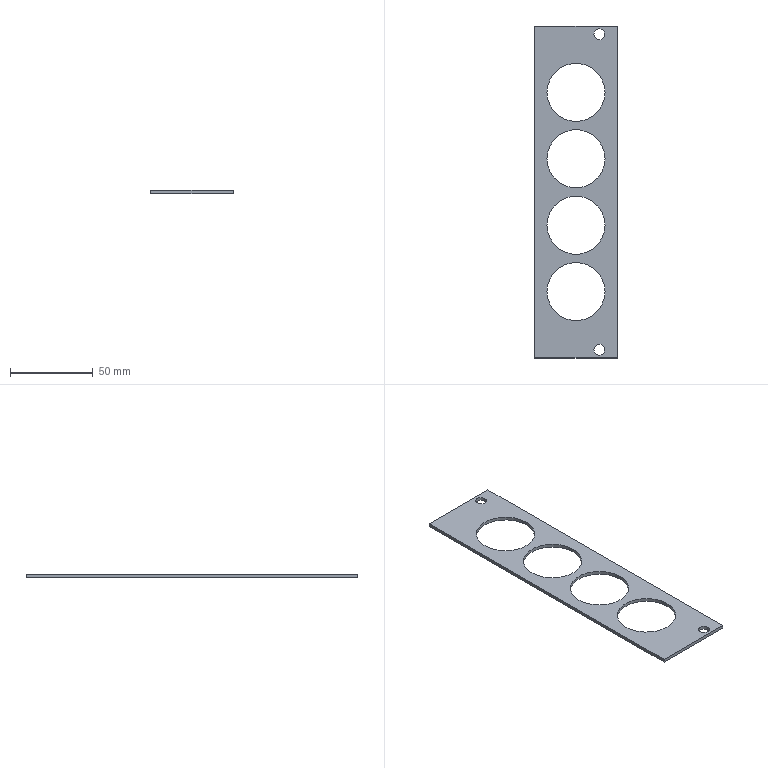Part | SolidWorks | features BaseBody 1 | 1 solid | 18 faces | box 50 x 200 x 2 mm | volume 12170 mm3 | cylinder 12 | plane 6 | commonest cylinder face diameters 35 x8 6.5 x4
STEP:
#1=CARTESIAN_POINT('',(175.446,-4210.973,117.471));
#2=VERTEX_POINT('',#1);
#3=CARTESIAN_POINT('',(210.446,-4210.973,117.471));
#4=VERTEX_POINT('',#3);
#5=CARTESIAN_POINT('',(192.946,-4210.973,117.471));
#6=DIRECTION('',(0.,0.,1.));
#7=DIRECTION('',(1.,0.,0.));
#8=AXIS2_PLACEMENT_3D('',#5,#6,#7);
#9=CIRCLE('',#8,17.5);
#10=EDGE_CURVE('',#2,#4,#9,.T.);
#11=ORIENTED_EDGE('',*,*,#10,.F.);
#12=CARTESIAN_POINT('',(175.446,-4210.973,119.471));
#13=VERTEX_POINT('',#12);
#14=CARTESIAN_POINT('',(175.446,-4210.973,120.383));
#15=DIRECTION('',(0.,0.,1.));
#16=VECTOR('',#15,1000.);
#17=LINE('',#14,#16);
#18=EDGE_CURVE('',#2,#13,#17,.T.);
#19=ORIENTED_EDGE('',*,*,#18,.T.);
#20=CARTESIAN_POINT('',(210.446,-4210.973,119.471));
#21=VERTEX_POINT('',#20);
#22=CARTESIAN_POINT('',(192.946,-4210.973,119.471));
#23=DIRECTION('',(0.,0.,-1.));
#24=DIRECTION('',(1.,0.,0.));
#25=AXIS2_PLACEMENT_3D('',#22,#23,#24);
#26=CIRCLE('',#25,17.5);
#27=EDGE_CURVE('',#21,#13,#26,.T.);
#28=ORIENTED_EDGE('',*,*,#27,.F.);
#29=CARTESIAN_POINT('',(210.446,-4210.973,120.383));
#30=DIRECTION('',(0.,0.,1.));
#31=VECTOR('',#30,1000.);
#32=LINE('',#29,#31);
#33=EDGE_CURVE('',#4,#21,#32,.T.);
#34=ORIENTED_EDGE('',*,*,#33,.F.);
#35=EDGE_LOOP('',(#11,#19,#28,#34));
#36=FACE_OUTER_BOUND('',#35,.T.);
#37=CARTESIAN_POINT('',(192.946,-4210.973,120.383));
#38=DIRECTION('',(0.,0.,1.));
#39=DIRECTION('',(1.,0.,0.));
#40=AXIS2_PLACEMENT_3D('',#37,#38,#39);
#41=CYLINDRICAL_SURFACE('',#40,17.5);
#42=ADVANCED_FACE('',(#36),#41,.F.);
#43=CARTESIAN_POINT('',(210.446,-4250.973,119.471));
#44=VERTEX_POINT('',#43);
#45=CARTESIAN_POINT('',(175.446,-4250.973,119.471));
#46=VERTEX_POINT('',#45);
#47=CARTESIAN_POINT('',(192.946,-4250.973,119.471));
#48=DIRECTION('',(0.,0.,-1.));
#49=DIRECTION('',(-1.,0.,0.));
#50=AXIS2_PLACEMENT_3D('',#47,#48,#49);
#51=CIRCLE('',#50,17.5);
#52=EDGE_CURVE('',#44,#46,#51,.T.);
#53=ORIENTED_EDGE('',*,*,#52,.F.);
#54=CARTESIAN_POINT('',(210.446,-4250.973,117.471));
#55=VERTEX_POINT('',#54);
#56=CARTESIAN_POINT('',(210.446,-4250.973,120.383));
#57=DIRECTION('',(0.,0.,-1.));
#58=VECTOR('',#57,1000.);
#59=LINE('',#56,#58);
#60=EDGE_CURVE('',#44,#55,#59,.T.);
#61=ORIENTED_EDGE('',*,*,#60,.T.);
#62=CARTESIAN_POINT('',(175.446,-4250.973,117.471));
#63=VERTEX_POINT('',#62);
#64=CARTESIAN_POINT('',(192.946,-4250.973,117.471));
#65=DIRECTION('',(0.,0.,1.));
#66=DIRECTION('',(-1.,0.,0.));
#67=AXIS2_PLACEMENT_3D('',#64,#65,#66);
#68=CIRCLE('',#67,17.5);
#69=EDGE_CURVE('',#63,#55,#68,.T.);
#70=ORIENTED_EDGE('',*,*,#69,.F.);
#71=CARTESIAN_POINT('',(175.446,-4250.973,120.383));
#72=DIRECTION('',(0.,0.,-1.));
#73=VECTOR('',#72,1000.);
#74=LINE('',#71,#73);
#75=EDGE_CURVE('',#46,#63,#74,.T.);
#76=ORIENTED_EDGE('',*,*,#75,.F.);
#77=EDGE_LOOP('',(#53,#61,#70,#76));
#78=FACE_OUTER_BOUND('',#77,.T.);
#79=CARTESIAN_POINT('',(192.946,-4250.973,120.383));
#80=DIRECTION('',(0.,0.,-1.));
#81=DIRECTION('',(-1.,0.,0.));
#82=AXIS2_PLACEMENT_3D('',#79,#80,#81);
#83=CYLINDRICAL_SURFACE('',#82,17.5);
#84=ADVANCED_FACE('',(#78),#83,.F.);
#85=CARTESIAN_POINT('',(203.696,-4135.973,117.471));
#86=VERTEX_POINT('',#85);
#87=CARTESIAN_POINT('',(210.196,-4135.973,117.471));
#88=VERTEX_POINT('',#87);
#89=CARTESIAN_POINT('',(206.946,-4135.973,117.471));
#90=DIRECTION('',(0.,0.,1.));
#91=DIRECTION('',(1.,0.,0.));
#92=AXIS2_PLACEMENT_3D('',#89,#90,#91);
#93=CIRCLE('',#92,3.25);
#94=EDGE_CURVE('',#86,#88,#93,.T.);
#95=ORIENTED_EDGE('',*,*,#94,.F.);
#96=CARTESIAN_POINT('',(203.696,-4135.973,119.471));
#97=VERTEX_POINT('',#96);
#98=CARTESIAN_POINT('',(203.696,-4135.973,120.383));
#99=DIRECTION('',(0.,0.,1.));
#100=VECTOR('',#99,1000.);
#101=LINE('',#98,#100);
#102=EDGE_CURVE('',#86,#97,#101,.T.);
#103=ORIENTED_EDGE('',*,*,#102,.T.);
#104=CARTESIAN_POINT('',(210.196,-4135.973,119.471));
#105=VERTEX_POINT('',#104);
#106=CARTESIAN_POINT('',(206.946,-4135.973,119.471));
#107=DIRECTION('',(0.,0.,-1.));
#108=DIRECTION('',(1.,0.,0.));
#109=AXIS2_PLACEMENT_3D('',#106,#107,#108);
#110=CIRCLE('',#109,3.25);
#111=EDGE_CURVE('',#105,#97,#110,.T.);
#112=ORIENTED_EDGE('',*,*,#111,.F.);
#113=CARTESIAN_POINT('',(210.196,-4135.973,120.383));
#114=DIRECTION('',(0.,0.,1.));
#115=VECTOR('',#114,1000.);
#116=LINE('',#113,#115);
#117=EDGE_CURVE('',#88,#105,#116,.T.);
#118=ORIENTED_EDGE('',*,*,#117,.F.);
#119=EDGE_LOOP('',(#95,#103,#112,#118));
#120=FACE_OUTER_BOUND('',#119,.T.);
#121=CARTESIAN_POINT('',(206.946,-4135.973,120.383));
#122=DIRECTION('',(0.,0.,1.));
#123=DIRECTION('',(1.,0.,0.));
#124=AXIS2_PLACEMENT_3D('',#121,#122,#123);
#125=CYLINDRICAL_SURFACE('',#124,3.25);
#126=ADVANCED_FACE('',(#120),#125,.F.);
#127=CARTESIAN_POINT('',(210.196,-4325.973,119.471));
#128=VERTEX_POINT('',#127);
#129=CARTESIAN_POINT('',(203.696,-4325.973,119.471));
#130=VERTEX_POINT('',#129);
#131=CARTESIAN_POINT('',(206.946,-4325.973,119.471));
#132=DIRECTION('',(0.,0.,-1.));
#133=DIRECTION('',(-1.,0.,0.));
#134=AXIS2_PLACEMENT_3D('',#131,#132,#133);
#135=CIRCLE('',#134,3.25);
#136=EDGE_CURVE('',#128,#130,#135,.T.);
#137=ORIENTED_EDGE('',*,*,#136,.F.);
#138=CARTESIAN_POINT('',(210.196,-4325.973,117.471));
#139=VERTEX_POINT('',#138);
#140=CARTESIAN_POINT('',(210.196,-4325.973,120.383));
#141=DIRECTION('',(0.,0.,-1.));
#142=VECTOR('',#141,1000.);
#143=LINE('',#140,#142);
#144=EDGE_CURVE('',#128,#139,#143,.T.);
#145=ORIENTED_EDGE('',*,*,#144,.T.);
#146=CARTESIAN_POINT('',(203.696,-4325.973,117.471));
#147=VERTEX_POINT('',#146);
#148=CARTESIAN_POINT('',(206.946,-4325.973,117.471));
#149=DIRECTION('',(0.,0.,1.));
#150=DIRECTION('',(-1.,0.,0.));
#151=AXIS2_PLACEMENT_3D('',#148,#149,#150);
#152=CIRCLE('',#151,3.25);
#153=EDGE_CURVE('',#147,#139,#152,.T.);
#154=ORIENTED_EDGE('',*,*,#153,.F.);
#155=CARTESIAN_POINT('',(203.696,-4325.973,120.383));
#156=DIRECTION('',(0.,0.,-1.));
#157=VECTOR('',#156,1000.);
#158=LINE('',#155,#157);
#159=EDGE_CURVE('',#130,#147,#158,.T.);
#160=ORIENTED_EDGE('',*,*,#159,.F.);
#161=EDGE_LOOP('',(#137,#145,#154,#160));
#162=FACE_OUTER_BOUND('',#161,.T.);
#163=CARTESIAN_POINT('',(206.946,-4325.973,120.383));
#164=DIRECTION('',(0.,0.,-1.));
#165=DIRECTION('',(-1.,0.,0.));
#166=AXIS2_PLACEMENT_3D('',#163,#164,#165);
#167=CYLINDRICAL_SURFACE('',#166,3.25);
#168=ADVANCED_FACE('',(#162),#167,.F.);
#169=CARTESIAN_POINT('',(210.446,-4290.973,119.471));
#170=VERTEX_POINT('',#169);
#171=CARTESIAN_POINT('',(175.446,-4290.973,119.471));
#172=VERTEX_POINT('',#171);
#173=CARTESIAN_POINT('',(192.946,-4290.973,119.471));
#174=DIRECTION('',(0.,0.,-1.));
#175=DIRECTION('',(-1.,0.,0.));
#176=AXIS2_PLACEMENT_3D('',#173,#174,#175);
#177=CIRCLE('',#176,17.5);
#178=EDGE_CURVE('',#170,#172,#177,.T.);
#179=ORIENTED_EDGE('',*,*,#178,.F.);
#180=CARTESIAN_POINT('',(210.446,-4290.973,117.471));
#181=VERTEX_POINT('',#180);
#182=CARTESIAN_POINT('',(210.446,-4290.973,120.383));
#183=DIRECTION('',(0.,0.,-1.));
#184=VECTOR('',#183,1000.);
#185=LINE('',#182,#184);
#186=EDGE_CURVE('',#170,#181,#185,.T.);
#187=ORIENTED_EDGE('',*,*,#186,.T.);
#188=CARTESIAN_POINT('',(175.446,-4290.973,117.471));
#189=VERTEX_POINT('',#188);
#190=CARTESIAN_POINT('',(192.946,-4290.973,117.471));
#191=DIRECTION('',(0.,0.,1.));
#192=DIRECTION('',(-1.,0.,0.));
#193=AXIS2_PLACEMENT_3D('',#190,#191,#192);
#194=CIRCLE('',#193,17.5);
#195=EDGE_CURVE('',#189,#181,#194,.T.);
#196=ORIENTED_EDGE('',*,*,#195,.F.);
#197=CARTESIAN_POINT('',(175.446,-4290.973,120.383));
#198=DIRECTION('',(0.,0.,-1.));
#199=VECTOR('',#198,1000.);
#200=LINE('',#197,#199);
#201=EDGE_CURVE('',#172,#189,#200,.T.);
#202=ORIENTED_EDGE('',*,*,#201,.F.);
#203=EDGE_LOOP('',(#179,#187,#196,#202));
#204=FACE_OUTER_BOUND('',#203,.T.);
#205=CARTESIAN_POINT('',(192.946,-4290.973,120.383));
#206=DIRECTION('',(0.,0.,-1.));
#207=DIRECTION('',(-1.,0.,0.));
#208=AXIS2_PLACEMENT_3D('',#205,#206,#207);
#209=CYLINDRICAL_SURFACE('',#208,17.5);
#210=ADVANCED_FACE('',(#204),#209,.F.);
#211=CARTESIAN_POINT('',(175.446,-4170.973,117.471));
#212=VERTEX_POINT('',#211);
#213=CARTESIAN_POINT('',(210.446,-4170.973,117.471));
#214=VERTEX_POINT('',#213);
#215=CARTESIAN_POINT('',(192.946,-4170.973,117.471));
#216=DIRECTION('',(0.,0.,1.));
#217=DIRECTION('',(1.,0.,0.));
#218=AXIS2_PLACEMENT_3D('',#215,#216,#217);
#219=CIRCLE('',#218,17.5);
#220=EDGE_CURVE('',#212,#214,#219,.T.);
#221=ORIENTED_EDGE('',*,*,#220,.F.);
#222=CARTESIAN_POINT('',(175.446,-4170.973,119.471));
#223=VERTEX_POINT('',#222);
#224=CARTESIAN_POINT('',(175.446,-4170.973,120.383));
#225=DIRECTION('',(0.,0.,1.));
#226=VECTOR('',#225,1000.);
#227=LINE('',#224,#226);
#228=EDGE_CURVE('',#212,#223,#227,.T.);
#229=ORIENTED_EDGE('',*,*,#228,.T.);
#230=CARTESIAN_POINT('',(210.446,-4170.973,119.471));
#231=VERTEX_POINT('',#230);
#232=CARTESIAN_POINT('',(192.946,-4170.973,119.471));
#233=DIRECTION('',(0.,0.,-1.));
#234=DIRECTION('',(1.,0.,0.));
#235=AXIS2_PLACEMENT_3D('',#232,#233,#234);
#236=CIRCLE('',#235,17.5);
#237=EDGE_CURVE('',#231,#223,#236,.T.);
#238=ORIENTED_EDGE('',*,*,#237,.F.);
#239=CARTESIAN_POINT('',(210.446,-4170.973,120.383));
#240=DIRECTION('',(0.,0.,1.));
#241=VECTOR('',#240,1000.);
#242=LINE('',#239,#241);
#243=EDGE_CURVE('',#214,#231,#242,.T.);
#244=ORIENTED_EDGE('',*,*,#243,.F.);
#245=EDGE_LOOP('',(#221,#229,#238,#244));
#246=FACE_OUTER_BOUND('',#245,.T.);
#247=CARTESIAN_POINT('',(192.946,-4170.973,120.383));
#248=DIRECTION('',(0.,0.,1.));
#249=DIRECTION('',(1.,0.,0.));
#250=AXIS2_PLACEMENT_3D('',#247,#248,#249);
#251=CYLINDRICAL_SURFACE('',#250,17.5);
#252=ADVANCED_FACE('',(#246),#251,.F.);
#253=CARTESIAN_POINT('',(167.946,-4330.973,119.471));
#254=VERTEX_POINT('',#253);
#255=CARTESIAN_POINT('',(217.946,-4330.973,119.471));
#256=VERTEX_POINT('',#255);
#257=CARTESIAN_POINT('',(192.946,-4330.973,119.471));
#258=DIRECTION('',(1.,0.,0.));
#259=VECTOR('',#258,1000.);
#260=LINE('',#257,#259);
#261=EDGE_CURVE('',#254,#256,#260,.T.);
#262=ORIENTED_EDGE('',*,*,#261,.T.);
#263=CARTESIAN_POINT('',(217.946,-4130.973,119.471));
#264=VERTEX_POINT('',#263);
#265=CARTESIAN_POINT('',(217.946,-4230.973,119.471));
#266=DIRECTION('',(0.,1.,0.));
#267=VECTOR('',#266,1000.);
#268=LINE('',#265,#267);
#269=EDGE_CURVE('',#256,#264,#268,.T.);
#270=ORIENTED_EDGE('',*,*,#269,.T.);
#271=CARTESIAN_POINT('',(167.946,-4130.973,119.471));
#272=VERTEX_POINT('',#271);
#273=CARTESIAN_POINT('',(192.946,-4130.973,119.471));
#274=DIRECTION('',(-1.,0.,0.));
#275=VECTOR('',#274,1000.);
#276=LINE('',#273,#275);
#277=EDGE_CURVE('',#264,#272,#276,.T.);
#278=ORIENTED_EDGE('',*,*,#277,.T.);
#279=CARTESIAN_POINT('',(167.946,-4230.973,119.471));
#280=DIRECTION('',(0.,-1.,0.));
#281=VECTOR('',#280,1000.);
#282=LINE('',#279,#281);
#283=EDGE_CURVE('',#272,#254,#282,.T.);
#284=ORIENTED_EDGE('',*,*,#283,.T.);
#285=EDGE_LOOP('',(#262,#270,#278,#284));
#286=FACE_OUTER_BOUND('',#285,.T.);
#287=ORIENTED_EDGE('',*,*,#27,.T.);
#288=CARTESIAN_POINT('',(192.946,-4210.973,119.471));
#289=DIRECTION('',(0.,0.,-1.));
#290=DIRECTION('',(1.,0.,0.));
#291=AXIS2_PLACEMENT_3D('',#288,#289,#290);
#292=CIRCLE('',#291,17.5);
#293=EDGE_CURVE('',#13,#21,#292,.T.);
#294=ORIENTED_EDGE('',*,*,#293,.T.);
#295=EDGE_LOOP('',(#287,#294));
#296=FACE_BOUND('',#295,.T.);
#297=CARTESIAN_POINT('',(192.946,-4250.973,119.471));
#298=DIRECTION('',(0.,0.,-1.));
#299=DIRECTION('',(-1.,0.,0.));
#300=AXIS2_PLACEMENT_3D('',#297,#298,#299);
#301=CIRCLE('',#300,17.5);
#302=EDGE_CURVE('',#46,#44,#301,.T.);
#303=ORIENTED_EDGE('',*,*,#302,.T.);
#304=ORIENTED_EDGE('',*,*,#52,.T.);
#305=EDGE_LOOP('',(#303,#304));
#306=FACE_BOUND('',#305,.T.);
#307=ORIENTED_EDGE('',*,*,#111,.T.);
#308=CARTESIAN_POINT('',(206.946,-4135.973,119.471));
#309=DIRECTION('',(0.,0.,-1.));
#310=DIRECTION('',(1.,0.,0.));
#311=AXIS2_PLACEMENT_3D('',#308,#309,#310);
#312=CIRCLE('',#311,3.25);
#313=EDGE_CURVE('',#97,#105,#312,.T.);
#314=ORIENTED_EDGE('',*,*,#313,.T.);
#315=EDGE_LOOP('',(#307,#314));
#316=FACE_BOUND('',#315,.T.);
#317=CARTESIAN_POINT('',(206.946,-4325.973,119.471));
#318=DIRECTION('',(0.,0.,-1.));
#319=DIRECTION('',(-1.,0.,0.));
#320=AXIS2_PLACEMENT_3D('',#317,#318,#319);
#321=CIRCLE('',#320,3.25);
#322=EDGE_CURVE('',#130,#128,#321,.T.);
#323=ORIENTED_EDGE('',*,*,#322,.T.);
#324=ORIENTED_EDGE('',*,*,#136,.T.);
#325=EDGE_LOOP('',(#323,#324));
#326=FACE_BOUND('',#325,.T.);
#327=CARTESIAN_POINT('',(192.946,-4290.973,119.471));
#328=DIRECTION('',(0.,0.,-1.));
#329=DIRECTION('',(-1.,0.,0.));
#330=AXIS2_PLACEMENT_3D('',#327,#328,#329);
#331=CIRCLE('',#330,17.5);
#332=EDGE_CURVE('',#172,#170,#331,.T.);
#333=ORIENTED_EDGE('',*,*,#332,.T.);
#334=ORIENTED_EDGE('',*,*,#178,.T.);
#335=EDGE_LOOP('',(#333,#334));
#336=FACE_BOUND('',#335,.T.);
#337=ORIENTED_EDGE('',*,*,#237,.T.);
#338=CARTESIAN_POINT('',(192.946,-4170.973,119.471));
#339=DIRECTION('',(0.,0.,-1.));
#340=DIRECTION('',(1.,0.,0.));
#341=AXIS2_PLACEMENT_3D('',#338,#339,#340);
#342=CIRCLE('',#341,17.5);
#343=EDGE_CURVE('',#223,#231,#342,.T.);
#344=ORIENTED_EDGE('',*,*,#343,.T.);
#345=EDGE_LOOP('',(#337,#344));
#346=FACE_BOUND('',#345,.T.);
#347=CARTESIAN_POINT('',(192.946,-4230.973,119.471));
#348=DIRECTION('',(0.,0.,1.));
#349=DIRECTION('',(1.,0.,0.));
#350=AXIS2_PLACEMENT_3D('',#347,#348,#349);
#351=PLANE('',#350);
#352=ADVANCED_FACE('',(#286,#296,#306,#316,#326,#336,#346),#351,.T.);
#353=CARTESIAN_POINT('',(217.946,-4330.973,117.471));
#354=VERTEX_POINT('',#353);
#355=CARTESIAN_POINT('',(217.946,-4130.973,117.471));
#356=VERTEX_POINT('',#355);
#357=CARTESIAN_POINT('',(217.946,-4130.973,117.471));
#358=DIRECTION('',(0.,1.,0.));
#359=VECTOR('',#358,1000.);
#360=LINE('',#357,#359);
#361=EDGE_CURVE('',#354,#356,#360,.T.);
#362=ORIENTED_EDGE('',*,*,#361,.T.);
#363=CARTESIAN_POINT('',(217.946,-4130.973,117.471));
#364=DIRECTION('',(0.,0.,1.));
#365=VECTOR('',#364,1000.);
#366=LINE('',#363,#365);
#367=EDGE_CURVE('',#356,#264,#366,.T.);
#368=ORIENTED_EDGE('',*,*,#367,.T.);
#369=ORIENTED_EDGE('',*,*,#269,.F.);
#370=CARTESIAN_POINT('',(217.946,-4330.973,117.471));
#371=DIRECTION('',(0.,0.,-1.));
#372=VECTOR('',#371,1000.);
#373=LINE('',#370,#372);
#374=EDGE_CURVE('',#256,#354,#373,.T.);
#375=ORIENTED_EDGE('',*,*,#374,.T.);
#376=EDGE_LOOP('',(#362,#368,#369,#375));
#377=FACE_OUTER_BOUND('',#376,.T.);
#378=CARTESIAN_POINT('',(217.946,-4130.973,117.471));
#379=DIRECTION('',(1.,0.,0.));
#380=DIRECTION('',(0.,0.,-1.));
#381=AXIS2_PLACEMENT_3D('',#378,#379,#380);
#382=PLANE('',#381);
#383=ADVANCED_FACE('',(#377),#382,.T.);
#384=CARTESIAN_POINT('',(167.946,-4330.973,117.471));
#385=VERTEX_POINT('',#384);
#386=CARTESIAN_POINT('',(217.946,-4330.973,117.471));
#387=DIRECTION('',(1.,0.,0.));
#388=VECTOR('',#387,1000.);
#389=LINE('',#386,#388);
#390=EDGE_CURVE('',#385,#354,#389,.T.);
#391=ORIENTED_EDGE('',*,*,#390,.T.);
#392=ORIENTED_EDGE('',*,*,#374,.F.);
#393=ORIENTED_EDGE('',*,*,#261,.F.);
#394=CARTESIAN_POINT('',(167.946,-4330.973,117.471));
#395=DIRECTION('',(0.,0.,-1.));
#396=VECTOR('',#395,1000.);
#397=LINE('',#394,#396);
#398=EDGE_CURVE('',#254,#385,#397,.T.);
#399=ORIENTED_EDGE('',*,*,#398,.T.);
#400=EDGE_LOOP('',(#391,#392,#393,#399));
#401=FACE_OUTER_BOUND('',#400,.T.);
#402=CARTESIAN_POINT('',(217.946,-4330.973,117.471));
#403=DIRECTION('',(0.,-1.,0.));
#404=DIRECTION('',(0.,0.,-1.));
#405=AXIS2_PLACEMENT_3D('',#402,#403,#404);
#406=PLANE('',#405);
#407=ADVANCED_FACE('',(#401),#406,.T.);
#408=CARTESIAN_POINT('',(167.946,-4130.973,117.471));
#409=VERTEX_POINT('',#408);
#410=CARTESIAN_POINT('',(167.946,-4330.973,117.471));
#411=DIRECTION('',(0.,-1.,0.));
#412=VECTOR('',#411,1000.);
#413=LINE('',#410,#412);
#414=EDGE_CURVE('',#409,#385,#413,.T.);
#415=ORIENTED_EDGE('',*,*,#414,.T.);
#416=ORIENTED_EDGE('',*,*,#398,.F.);
#417=ORIENTED_EDGE('',*,*,#283,.F.);
#418=CARTESIAN_POINT('',(167.946,-4130.973,117.471));
#419=DIRECTION('',(0.,0.,-1.));
#420=VECTOR('',#419,1000.);
#421=LINE('',#418,#420);
#422=EDGE_CURVE('',#272,#409,#421,.T.);
#423=ORIENTED_EDGE('',*,*,#422,.T.);
#424=EDGE_LOOP('',(#415,#416,#417,#423));
#425=FACE_OUTER_BOUND('',#424,.T.);
#426=CARTESIAN_POINT('',(167.946,-4330.973,117.471));
#427=DIRECTION('',(-1.,0.,0.));
#428=DIRECTION('',(0.,0.,1.));
#429=AXIS2_PLACEMENT_3D('',#426,#427,#428);
#430=PLANE('',#429);
#431=ADVANCED_FACE('',(#425),#430,.T.);
#432=CARTESIAN_POINT('',(167.946,-4130.973,117.471));
#433=DIRECTION('',(-1.,0.,0.));
#434=VECTOR('',#433,1000.);
#435=LINE('',#432,#434);
#436=EDGE_CURVE('',#356,#409,#435,.T.);
#437=ORIENTED_EDGE('',*,*,#436,.T.);
#438=ORIENTED_EDGE('',*,*,#422,.F.);
#439=ORIENTED_EDGE('',*,*,#277,.F.);
#440=ORIENTED_EDGE('',*,*,#367,.F.);
#441=EDGE_LOOP('',(#437,#438,#439,#440));
#442=FACE_OUTER_BOUND('',#441,.T.);
#443=CARTESIAN_POINT('',(167.946,-4130.973,117.471));
#444=DIRECTION('',(0.,1.,0.));
#445=DIRECTION('',(0.,0.,1.));
#446=AXIS2_PLACEMENT_3D('',#443,#444,#445);
#447=PLANE('',#446);
#448=ADVANCED_FACE('',(#442),#447,.T.);
#449=ORIENTED_EDGE('',*,*,#18,.F.);
#450=CARTESIAN_POINT('',(192.946,-4210.973,117.471));
#451=DIRECTION('',(0.,0.,1.));
#452=DIRECTION('',(1.,0.,0.));
#453=AXIS2_PLACEMENT_3D('',#450,#451,#452);
#454=CIRCLE('',#453,17.5);
#455=EDGE_CURVE('',#4,#2,#454,.T.);
#456=ORIENTED_EDGE('',*,*,#455,.F.);
#457=ORIENTED_EDGE('',*,*,#33,.T.);
#458=ORIENTED_EDGE('',*,*,#293,.F.);
#459=EDGE_LOOP('',(#449,#456,#457,#458));
#460=FACE_OUTER_BOUND('',#459,.T.);
#461=CARTESIAN_POINT('',(192.946,-4210.973,120.383));
#462=DIRECTION('',(0.,0.,1.));
#463=DIRECTION('',(1.,0.,0.));
#464=AXIS2_PLACEMENT_3D('',#461,#462,#463);
#465=CYLINDRICAL_SURFACE('',#464,17.5);
#466=ADVANCED_FACE('',(#460),#465,.F.);
#467=ORIENTED_EDGE('',*,*,#60,.F.);
#468=ORIENTED_EDGE('',*,*,#302,.F.);
#469=ORIENTED_EDGE('',*,*,#75,.T.);
#470=CARTESIAN_POINT('',(192.946,-4250.973,117.471));
#471=DIRECTION('',(0.,0.,1.));
#472=DIRECTION('',(-1.,0.,0.));
#473=AXIS2_PLACEMENT_3D('',#470,#471,#472);
#474=CIRCLE('',#473,17.5);
#475=EDGE_CURVE('',#55,#63,#474,.T.);
#476=ORIENTED_EDGE('',*,*,#475,.F.);
#477=EDGE_LOOP('',(#467,#468,#469,#476));
#478=FACE_OUTER_BOUND('',#477,.T.);
#479=CARTESIAN_POINT('',(192.946,-4250.973,120.383));
#480=DIRECTION('',(0.,0.,-1.));
#481=DIRECTION('',(-1.,0.,0.));
#482=AXIS2_PLACEMENT_3D('',#479,#480,#481);
#483=CYLINDRICAL_SURFACE('',#482,17.5);
#484=ADVANCED_FACE('',(#478),#483,.F.);
#485=ORIENTED_EDGE('',*,*,#102,.F.);
#486=CARTESIAN_POINT('',(206.946,-4135.973,117.471));
#487=DIRECTION('',(0.,0.,1.));
#488=DIRECTION('',(1.,0.,0.));
#489=AXIS2_PLACEMENT_3D('',#486,#487,#488);
#490=CIRCLE('',#489,3.25);
#491=EDGE_CURVE('',#88,#86,#490,.T.);
#492=ORIENTED_EDGE('',*,*,#491,.F.);
#493=ORIENTED_EDGE('',*,*,#117,.T.);
#494=ORIENTED_EDGE('',*,*,#313,.F.);
#495=EDGE_LOOP('',(#485,#492,#493,#494));
#496=FACE_OUTER_BOUND('',#495,.T.);
#497=CARTESIAN_POINT('',(206.946,-4135.973,120.383));
#498=DIRECTION('',(0.,0.,1.));
#499=DIRECTION('',(1.,0.,0.));
#500=AXIS2_PLACEMENT_3D('',#497,#498,#499);
#501=CYLINDRICAL_SURFACE('',#500,3.25);
#502=ADVANCED_FACE('',(#496),#501,.F.);
#503=ORIENTED_EDGE('',*,*,#144,.F.);
#504=ORIENTED_EDGE('',*,*,#322,.F.);
#505=ORIENTED_EDGE('',*,*,#159,.T.);
#506=CARTESIAN_POINT('',(206.946,-4325.973,117.471));
#507=DIRECTION('',(0.,0.,1.));
#508=DIRECTION('',(-1.,0.,0.));
#509=AXIS2_PLACEMENT_3D('',#506,#507,#508);
#510=CIRCLE('',#509,3.25);
#511=EDGE_CURVE('',#139,#147,#510,.T.);
#512=ORIENTED_EDGE('',*,*,#511,.F.);
#513=EDGE_LOOP('',(#503,#504,#505,#512));
#514=FACE_OUTER_BOUND('',#513,.T.);
#515=CARTESIAN_POINT('',(206.946,-4325.973,120.383));
#516=DIRECTION('',(0.,0.,-1.));
#517=DIRECTION('',(-1.,0.,0.));
#518=AXIS2_PLACEMENT_3D('',#515,#516,#517);
#519=CYLINDRICAL_SURFACE('',#518,3.25);
#520=ADVANCED_FACE('',(#514),#519,.F.);
#521=ORIENTED_EDGE('',*,*,#186,.F.);
#522=ORIENTED_EDGE('',*,*,#332,.F.);
#523=ORIENTED_EDGE('',*,*,#201,.T.);
#524=CARTESIAN_POINT('',(192.946,-4290.973,117.471));
#525=DIRECTION('',(0.,0.,1.));
#526=DIRECTION('',(-1.,0.,0.));
#527=AXIS2_PLACEMENT_3D('',#524,#525,#526);
#528=CIRCLE('',#527,17.5);
#529=EDGE_CURVE('',#181,#189,#528,.T.);
#530=ORIENTED_EDGE('',*,*,#529,.F.);
#531=EDGE_LOOP('',(#521,#522,#523,#530));
#532=FACE_OUTER_BOUND('',#531,.T.);
#533=CARTESIAN_POINT('',(192.946,-4290.973,120.383));
#534=DIRECTION('',(0.,0.,-1.));
#535=DIRECTION('',(-1.,0.,0.));
#536=AXIS2_PLACEMENT_3D('',#533,#534,#535);
#537=CYLINDRICAL_SURFACE('',#536,17.5);
#538=ADVANCED_FACE('',(#532),#537,.F.);
#539=ORIENTED_EDGE('',*,*,#228,.F.);
#540=CARTESIAN_POINT('',(192.946,-4170.973,117.471));
#541=DIRECTION('',(0.,0.,1.));
#542=DIRECTION('',(1.,0.,0.));
#543=AXIS2_PLACEMENT_3D('',#540,#541,#542);
#544=CIRCLE('',#543,17.5);
#545=EDGE_CURVE('',#214,#212,#544,.T.);
#546=ORIENTED_EDGE('',*,*,#545,.F.);
#547=ORIENTED_EDGE('',*,*,#243,.T.);
#548=ORIENTED_EDGE('',*,*,#343,.F.);
#549=EDGE_LOOP('',(#539,#546,#547,#548));
#550=FACE_OUTER_BOUND('',#549,.T.);
#551=CARTESIAN_POINT('',(192.946,-4170.973,120.383));
#552=DIRECTION('',(0.,0.,1.));
#553=DIRECTION('',(1.,0.,0.));
#554=AXIS2_PLACEMENT_3D('',#551,#552,#553);
#555=CYLINDRICAL_SURFACE('',#554,17.5);
#556=ADVANCED_FACE('',(#550),#555,.F.);
#557=ORIENTED_EDGE('',*,*,#436,.F.);
#558=ORIENTED_EDGE('',*,*,#361,.F.);
#559=ORIENTED_EDGE('',*,*,#390,.F.);
#560=ORIENTED_EDGE('',*,*,#414,.F.);
#561=EDGE_LOOP('',(#557,#558,#559,#560));
#562=FACE_OUTER_BOUND('',#561,.T.);
#563=ORIENTED_EDGE('',*,*,#455,.T.);
#564=ORIENTED_EDGE('',*,*,#10,.T.);
#565=EDGE_LOOP('',(#563,#564));
#566=FACE_BOUND('',#565,.T.);
#567=ORIENTED_EDGE('',*,*,#69,.T.);
#568=ORIENTED_EDGE('',*,*,#475,.T.);
#569=EDGE_LOOP('',(#567,#568));
#570=FACE_BOUND('',#569,.T.);
#571=ORIENTED_EDGE('',*,*,#491,.T.);
#572=ORIENTED_EDGE('',*,*,#94,.T.);
#573=EDGE_LOOP('',(#571,#572));
#574=FACE_BOUND('',#573,.T.);
#575=ORIENTED_EDGE('',*,*,#153,.T.);
#576=ORIENTED_EDGE('',*,*,#511,.T.);
#577=EDGE_LOOP('',(#575,#576));
#578=FACE_BOUND('',#577,.T.);
#579=ORIENTED_EDGE('',*,*,#195,.T.);
#580=ORIENTED_EDGE('',*,*,#529,.T.);
#581=EDGE_LOOP('',(#579,#580));
#582=FACE_BOUND('',#581,.T.);
#583=ORIENTED_EDGE('',*,*,#545,.T.);
#584=ORIENTED_EDGE('',*,*,#220,.T.);
#585=EDGE_LOOP('',(#583,#584));
#586=FACE_BOUND('',#585,.T.);
#587=CARTESIAN_POINT('',(192.946,-4230.973,117.471));
#588=DIRECTION('',(0.,0.,1.));
#589=DIRECTION('',(1.,0.,0.));
#590=AXIS2_PLACEMENT_3D('',#587,#588,#589);
#591=PLANE('',#590);
#592=ADVANCED_FACE('',(#562,#566,#570,#574,#578,#582,#586),#591,.F.);
#593=CLOSED_SHELL('',(#42,#84,#126,#168,#210,#252,#352,#383,#407,#431,#448,#466,#484,#502,#520,#538,#556,#592));
#594=MANIFOLD_SOLID_BREP('',#593);
#595=CARTESIAN_POINT('',(0.,0.,0.));
#596=DIRECTION('',(0.,0.,1.));
#597=DIRECTION('',(1.,0.,0.));
#598=AXIS2_PLACEMENT_3D('',#595,#596,#597);
#599=(LENGTH_UNIT()NAMED_UNIT(*)SI_UNIT(.MILLI.,.METRE.));
#600=UNCERTAINTY_MEASURE_WITH_UNIT(LENGTH_MEASURE(0.00001),#599,'','');
#601=(NAMED_UNIT(*)PLANE_ANGLE_UNIT()SI_UNIT($,.RADIAN.));
#602=(NAMED_UNIT(*)SI_UNIT($,.STERADIAN.)SOLID_ANGLE_UNIT());
#603=(GEOMETRIC_REPRESENTATION_CONTEXT(3)GLOBAL_UNCERTAINTY_ASSIGNED_CONTEXT((#600))GLOBAL_UNIT_ASSIGNED_CONTEXT((#599,#601,#602))REPRESENTATION_CONTEXT('',''));
#604=ADVANCED_BREP_SHAPE_REPRESENTATION('',(#594,#598),#603);